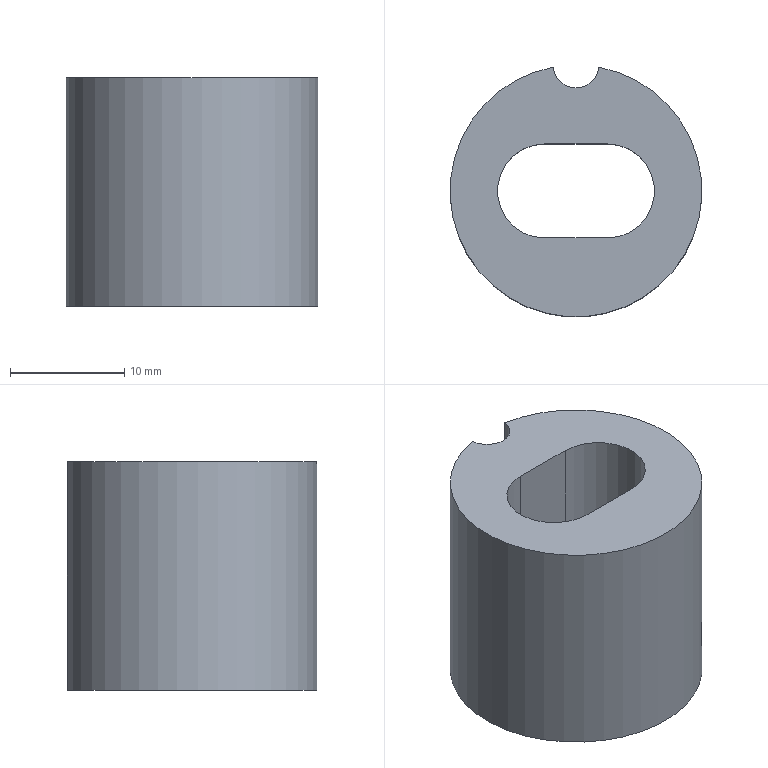Part | NX | features solid 2 | 1 solid | 10 faces | box 22 x 21.818 x 20 mm | volume 4687 mm3 | plane 5 | cylinder 5 | commonest cylinder face diameters 8.22 x2 4 x1 14.6 x1 22 x1
STEP:
#1=CARTESIAN_POINT('',(-66.242,23.158,-5.281));
#2=VERTEX_POINT('',#1);
#3=CARTESIAN_POINT('',(-70.226,23.158,-5.281));
#4=VERTEX_POINT('',#3);
#5=CARTESIAN_POINT('',(-68.234,23.34,-5.281));
#6=DIRECTION('',(0.,0.,-1.));
#7=DIRECTION('',(0.,-1.,0.));
#8=AXIS2_PLACEMENT_3D('',#5,#6,#7);
#9=CIRCLE('',#8,2.);
#10=EDGE_CURVE('',#2,#4,#9,.T.);
#11=ORIENTED_EDGE('',*,*,#10,.T.);
#12=CARTESIAN_POINT('',(-68.234,12.34,-5.281));
#13=DIRECTION('',(0.,0.,1.));
#14=DIRECTION('',(-1.,0.,0.));
#15=AXIS2_PLACEMENT_3D('',#12,#13,#14);
#16=CIRCLE('',#15,11.);
#17=EDGE_CURVE('',#2,#4,#16,.F.);
#18=ORIENTED_EDGE('',*,*,#17,.F.);
#19=EDGE_LOOP('',(#11,#18));
#20=FACE_BOUND('',#19,.T.);
#21=CARTESIAN_POINT('',(-70.984,8.23,-5.281));
#22=VERTEX_POINT('',#21);
#23=CARTESIAN_POINT('',(-70.984,16.45,-5.281));
#24=VERTEX_POINT('',#23);
#25=CARTESIAN_POINT('',(-70.984,12.34,-5.281));
#26=DIRECTION('',(0.,0.,-1.));
#27=DIRECTION('',(0.,-1.,0.));
#28=AXIS2_PLACEMENT_3D('',#25,#26,#27);
#29=CIRCLE('',#28,4.11);
#30=EDGE_CURVE('',#22,#24,#29,.T.);
#31=ORIENTED_EDGE('',*,*,#30,.T.);
#32=CARTESIAN_POINT('',(-65.484,16.45,-5.281));
#33=VERTEX_POINT('',#32);
#34=CARTESIAN_POINT('',(-68.234,16.45,-5.281));
#35=DIRECTION('',(1.,0.,0.));
#36=VECTOR('',#35,1000.);
#37=LINE('',#34,#36);
#38=EDGE_CURVE('',#24,#33,#37,.T.);
#39=ORIENTED_EDGE('',*,*,#38,.T.);
#40=CARTESIAN_POINT('',(-65.484,8.23,-5.281));
#41=VERTEX_POINT('',#40);
#42=CARTESIAN_POINT('',(-65.484,12.34,-5.281));
#43=DIRECTION('',(0.,0.,-1.));
#44=DIRECTION('',(0.,-1.,0.));
#45=AXIS2_PLACEMENT_3D('',#42,#43,#44);
#46=CIRCLE('',#45,4.11);
#47=EDGE_CURVE('',#33,#41,#46,.T.);
#48=ORIENTED_EDGE('',*,*,#47,.T.);
#49=CARTESIAN_POINT('',(-68.234,8.23,-5.281));
#50=DIRECTION('',(-1.,0.,0.));
#51=VECTOR('',#50,1000.);
#52=LINE('',#49,#51);
#53=EDGE_CURVE('',#41,#22,#52,.T.);
#54=ORIENTED_EDGE('',*,*,#53,.T.);
#55=EDGE_LOOP('',(#31,#39,#48,#54));
#56=FACE_BOUND('',#55,.T.);
#57=CARTESIAN_POINT('',(-68.234,12.34,-5.281));
#58=DIRECTION('',(0.,0.,1.));
#59=DIRECTION('',(0.,1.,0.));
#60=AXIS2_PLACEMENT_3D('',#57,#58,#59);
#61=PLANE('',#60);
#62=ADVANCED_FACE('',(#20,#56),#61,.T.);
#63=CARTESIAN_POINT('',(-70.226,23.158,-25.281));
#64=VERTEX_POINT('',#63);
#65=CARTESIAN_POINT('',(-66.242,23.158,-25.281));
#66=VERTEX_POINT('',#65);
#67=CARTESIAN_POINT('',(-68.234,23.34,-25.281));
#68=DIRECTION('',(0.,0.,1.));
#69=DIRECTION('',(0.,1.,0.));
#70=AXIS2_PLACEMENT_3D('',#67,#68,#69);
#71=CIRCLE('',#70,2.);
#72=EDGE_CURVE('',#64,#66,#71,.T.);
#73=ORIENTED_EDGE('',*,*,#72,.T.);
#74=CARTESIAN_POINT('',(-68.234,12.34,-25.281));
#75=DIRECTION('',(0.,0.,-1.));
#76=DIRECTION('',(1.,0.,0.));
#77=AXIS2_PLACEMENT_3D('',#74,#75,#76);
#78=CIRCLE('',#77,11.);
#79=EDGE_CURVE('',#64,#66,#78,.F.);
#80=ORIENTED_EDGE('',*,*,#79,.F.);
#81=EDGE_LOOP('',(#73,#80));
#82=FACE_BOUND('',#81,.T.);
#83=CARTESIAN_POINT('',(-75.534,12.34,-25.281));
#84=VERTEX_POINT('',#83);
#85=CARTESIAN_POINT('',(-68.234,12.34,-25.281));
#86=DIRECTION('',(0.,0.,-1.));
#87=DIRECTION('',(-1.,0.,0.));
#88=AXIS2_PLACEMENT_3D('',#85,#86,#87);
#89=CIRCLE('',#88,7.3);
#90=EDGE_CURVE('',#84,#84,#89,.F.);
#91=ORIENTED_EDGE('',*,*,#90,.T.);
#92=EDGE_LOOP('',(#91));
#93=FACE_BOUND('',#92,.T.);
#94=CARTESIAN_POINT('',(-68.234,12.34,-25.281));
#95=DIRECTION('',(0.,0.,-1.));
#96=DIRECTION('',(0.,-1.,0.));
#97=AXIS2_PLACEMENT_3D('',#94,#95,#96);
#98=PLANE('',#97);
#99=ADVANCED_FACE('',(#82,#93),#98,.T.);
#100=CARTESIAN_POINT('',(-70.226,23.158,-15.281));
#101=DIRECTION('',(0.,0.,1.));
#102=VECTOR('',#101,1000.);
#103=LINE('',#100,#102);
#104=EDGE_CURVE('',#64,#4,#103,.T.);
#105=ORIENTED_EDGE('',*,*,#104,.F.);
#106=ORIENTED_EDGE('',*,*,#79,.T.);
#107=CARTESIAN_POINT('',(-66.242,23.158,-15.281));
#108=DIRECTION('',(0.,0.,1.));
#109=VECTOR('',#108,1000.);
#110=LINE('',#107,#109);
#111=EDGE_CURVE('',#2,#66,#110,.F.);
#112=ORIENTED_EDGE('',*,*,#111,.F.);
#113=ORIENTED_EDGE('',*,*,#17,.T.);
#114=EDGE_LOOP('',(#105,#106,#112,#113));
#115=FACE_BOUND('',#114,.T.);
#116=CARTESIAN_POINT('',(-68.234,12.34,-25.281));
#117=DIRECTION('',(0.,0.,1.));
#118=DIRECTION('',(0.,1.,0.));
#119=AXIS2_PLACEMENT_3D('',#116,#117,#118);
#120=CYLINDRICAL_SURFACE('',#119,11.);
#121=ADVANCED_FACE('',(#115),#120,.T.);
#122=CARTESIAN_POINT('',(-65.484,16.45,-13.281));
#123=VERTEX_POINT('',#122);
#124=CARTESIAN_POINT('',(-70.984,16.45,-13.281));
#125=VERTEX_POINT('',#124);
#126=CARTESIAN_POINT('',(-68.234,16.45,-13.281));
#127=DIRECTION('',(-1.,0.,0.));
#128=VECTOR('',#127,1000.);
#129=LINE('',#126,#128);
#130=EDGE_CURVE('',#123,#125,#129,.T.);
#131=ORIENTED_EDGE('',*,*,#130,.T.);
#132=CARTESIAN_POINT('',(-70.984,8.23,-13.281));
#133=VERTEX_POINT('',#132);
#134=CARTESIAN_POINT('',(-70.984,12.34,-13.281));
#135=DIRECTION('',(0.,0.,1.));
#136=DIRECTION('',(0.,1.,0.));
#137=AXIS2_PLACEMENT_3D('',#134,#135,#136);
#138=CIRCLE('',#137,4.11);
#139=EDGE_CURVE('',#125,#133,#138,.T.);
#140=ORIENTED_EDGE('',*,*,#139,.T.);
#141=CARTESIAN_POINT('',(-65.484,8.23,-13.281));
#142=VERTEX_POINT('',#141);
#143=CARTESIAN_POINT('',(-68.234,8.23,-13.281));
#144=DIRECTION('',(1.,0.,0.));
#145=VECTOR('',#144,1000.);
#146=LINE('',#143,#145);
#147=EDGE_CURVE('',#133,#142,#146,.T.);
#148=ORIENTED_EDGE('',*,*,#147,.T.);
#149=CARTESIAN_POINT('',(-65.484,12.34,-13.281));
#150=DIRECTION('',(0.,0.,1.));
#151=DIRECTION('',(0.,1.,0.));
#152=AXIS2_PLACEMENT_3D('',#149,#150,#151);
#153=CIRCLE('',#152,4.11);
#154=EDGE_CURVE('',#142,#123,#153,.T.);
#155=ORIENTED_EDGE('',*,*,#154,.T.);
#156=EDGE_LOOP('',(#131,#140,#148,#155));
#157=FACE_BOUND('',#156,.T.);
#158=CARTESIAN_POINT('',(-60.934,12.34,-13.281));
#159=VERTEX_POINT('',#158);
#160=CARTESIAN_POINT('',(-68.234,12.34,-13.281));
#161=DIRECTION('',(0.,0.,1.));
#162=DIRECTION('',(1.,0.,0.));
#163=AXIS2_PLACEMENT_3D('',#160,#161,#162);
#164=CIRCLE('',#163,7.3);
#165=EDGE_CURVE('',#159,#159,#164,.F.);
#166=ORIENTED_EDGE('',*,*,#165,.T.);
#167=EDGE_LOOP('',(#166));
#168=FACE_BOUND('',#167,.T.);
#169=CARTESIAN_POINT('',(-68.234,12.34,-13.281));
#170=DIRECTION('',(0.,0.,1.));
#171=DIRECTION('',(0.,1.,0.));
#172=AXIS2_PLACEMENT_3D('',#169,#170,#171);
#173=PLANE('',#172);
#174=ADVANCED_FACE('',(#157,#168),#173,.F.);
#175=ORIENTED_EDGE('',*,*,#165,.F.);
#176=EDGE_LOOP('',(#175));
#177=FACE_BOUND('',#176,.T.);
#178=ORIENTED_EDGE('',*,*,#90,.F.);
#179=EDGE_LOOP('',(#178));
#180=FACE_BOUND('',#179,.T.);
#181=CARTESIAN_POINT('',(-68.234,12.34,-25.281));
#182=DIRECTION('',(0.,0.,1.));
#183=DIRECTION('',(0.,1.,0.));
#184=AXIS2_PLACEMENT_3D('',#181,#182,#183);
#185=CYLINDRICAL_SURFACE('',#184,7.3);
#186=ADVANCED_FACE('',(#177,#180),#185,.F.);
#187=CARTESIAN_POINT('',(-65.484,8.23,-13.281));
#188=DIRECTION('',(0.,0.,1.));
#189=VECTOR('',#188,1000.);
#190=LINE('',#187,#189);
#191=EDGE_CURVE('',#142,#41,#190,.T.);
#192=ORIENTED_EDGE('',*,*,#191,.F.);
#193=ORIENTED_EDGE('',*,*,#147,.F.);
#194=CARTESIAN_POINT('',(-70.984,8.23,-13.281));
#195=DIRECTION('',(0.,0.,1.));
#196=VECTOR('',#195,1000.);
#197=LINE('',#194,#196);
#198=EDGE_CURVE('',#133,#22,#197,.T.);
#199=ORIENTED_EDGE('',*,*,#198,.T.);
#200=ORIENTED_EDGE('',*,*,#53,.F.);
#201=EDGE_LOOP('',(#192,#193,#199,#200));
#202=FACE_BOUND('',#201,.T.);
#203=CARTESIAN_POINT('',(-68.234,8.23,-13.281));
#204=DIRECTION('',(0.,-1.,0.));
#205=DIRECTION('',(0.,0.,1.));
#206=AXIS2_PLACEMENT_3D('',#203,#204,#205);
#207=PLANE('',#206);
#208=ADVANCED_FACE('',(#202),#207,.F.);
#209=ORIENTED_EDGE('',*,*,#130,.F.);
#210=CARTESIAN_POINT('',(-65.484,16.45,-13.281));
#211=DIRECTION('',(0.,0.,1.));
#212=VECTOR('',#211,1000.);
#213=LINE('',#210,#212);
#214=EDGE_CURVE('',#123,#33,#213,.T.);
#215=ORIENTED_EDGE('',*,*,#214,.T.);
#216=ORIENTED_EDGE('',*,*,#38,.F.);
#217=CARTESIAN_POINT('',(-70.984,16.45,-13.281));
#218=DIRECTION('',(0.,0.,1.));
#219=VECTOR('',#218,1000.);
#220=LINE('',#217,#219);
#221=EDGE_CURVE('',#125,#24,#220,.T.);
#222=ORIENTED_EDGE('',*,*,#221,.F.);
#223=EDGE_LOOP('',(#209,#215,#216,#222));
#224=FACE_BOUND('',#223,.T.);
#225=CARTESIAN_POINT('',(-68.234,16.45,-13.281));
#226=DIRECTION('',(0.,1.,0.));
#227=DIRECTION('',(0.,0.,-1.));
#228=AXIS2_PLACEMENT_3D('',#225,#226,#227);
#229=PLANE('',#228);
#230=ADVANCED_FACE('',(#224),#229,.F.);
#231=ORIENTED_EDGE('',*,*,#191,.T.);
#232=ORIENTED_EDGE('',*,*,#47,.F.);
#233=ORIENTED_EDGE('',*,*,#214,.F.);
#234=ORIENTED_EDGE('',*,*,#154,.F.);
#235=EDGE_LOOP('',(#231,#232,#233,#234));
#236=FACE_BOUND('',#235,.T.);
#237=CARTESIAN_POINT('',(-65.484,12.34,-13.281));
#238=DIRECTION('',(0.,0.,1.));
#239=DIRECTION('',(0.,1.,0.));
#240=AXIS2_PLACEMENT_3D('',#237,#238,#239);
#241=CYLINDRICAL_SURFACE('',#240,4.11);
#242=ADVANCED_FACE('',(#236),#241,.F.);
#243=ORIENTED_EDGE('',*,*,#139,.F.);
#244=ORIENTED_EDGE('',*,*,#221,.T.);
#245=ORIENTED_EDGE('',*,*,#30,.F.);
#246=ORIENTED_EDGE('',*,*,#198,.F.);
#247=EDGE_LOOP('',(#243,#244,#245,#246));
#248=FACE_BOUND('',#247,.T.);
#249=CARTESIAN_POINT('',(-70.984,12.34,-13.281));
#250=DIRECTION('',(0.,0.,1.));
#251=DIRECTION('',(0.,1.,0.));
#252=AXIS2_PLACEMENT_3D('',#249,#250,#251);
#253=CYLINDRICAL_SURFACE('',#252,4.11);
#254=ADVANCED_FACE('',(#248),#253,.F.);
#255=ORIENTED_EDGE('',*,*,#104,.T.);
#256=ORIENTED_EDGE('',*,*,#10,.F.);
#257=ORIENTED_EDGE('',*,*,#111,.T.);
#258=ORIENTED_EDGE('',*,*,#72,.F.);
#259=EDGE_LOOP('',(#255,#256,#257,#258));
#260=FACE_BOUND('',#259,.T.);
#261=CARTESIAN_POINT('',(-68.234,23.34,-25.281));
#262=DIRECTION('',(0.,0.,1.));
#263=DIRECTION('',(0.,1.,0.));
#264=AXIS2_PLACEMENT_3D('',#261,#262,#263);
#265=CYLINDRICAL_SURFACE('',#264,2.);
#266=ADVANCED_FACE('',(#260),#265,.F.);
#267=CLOSED_SHELL('',(#62,#99,#121,#174,#186,#208,#230,#242,#254,#266));
#268=MANIFOLD_SOLID_BREP('',#267);
#269=(LENGTH_UNIT()NAMED_UNIT(*)SI_UNIT(.MILLI.,.METRE.));
#270=UNCERTAINTY_MEASURE_WITH_UNIT(LENGTH_MEASURE(0.00001),#269,'','');
#271=(NAMED_UNIT(*)PLANE_ANGLE_UNIT()SI_UNIT($,.RADIAN.));
#272=(NAMED_UNIT(*)SI_UNIT($,.STERADIAN.)SOLID_ANGLE_UNIT());
#273=(GEOMETRIC_REPRESENTATION_CONTEXT(3)GLOBAL_UNCERTAINTY_ASSIGNED_CONTEXT((#270))GLOBAL_UNIT_ASSIGNED_CONTEXT((#269,#271,#272))REPRESENTATION_CONTEXT('',''));
#274=ADVANCED_BREP_SHAPE_REPRESENTATION('',(#268),#273);